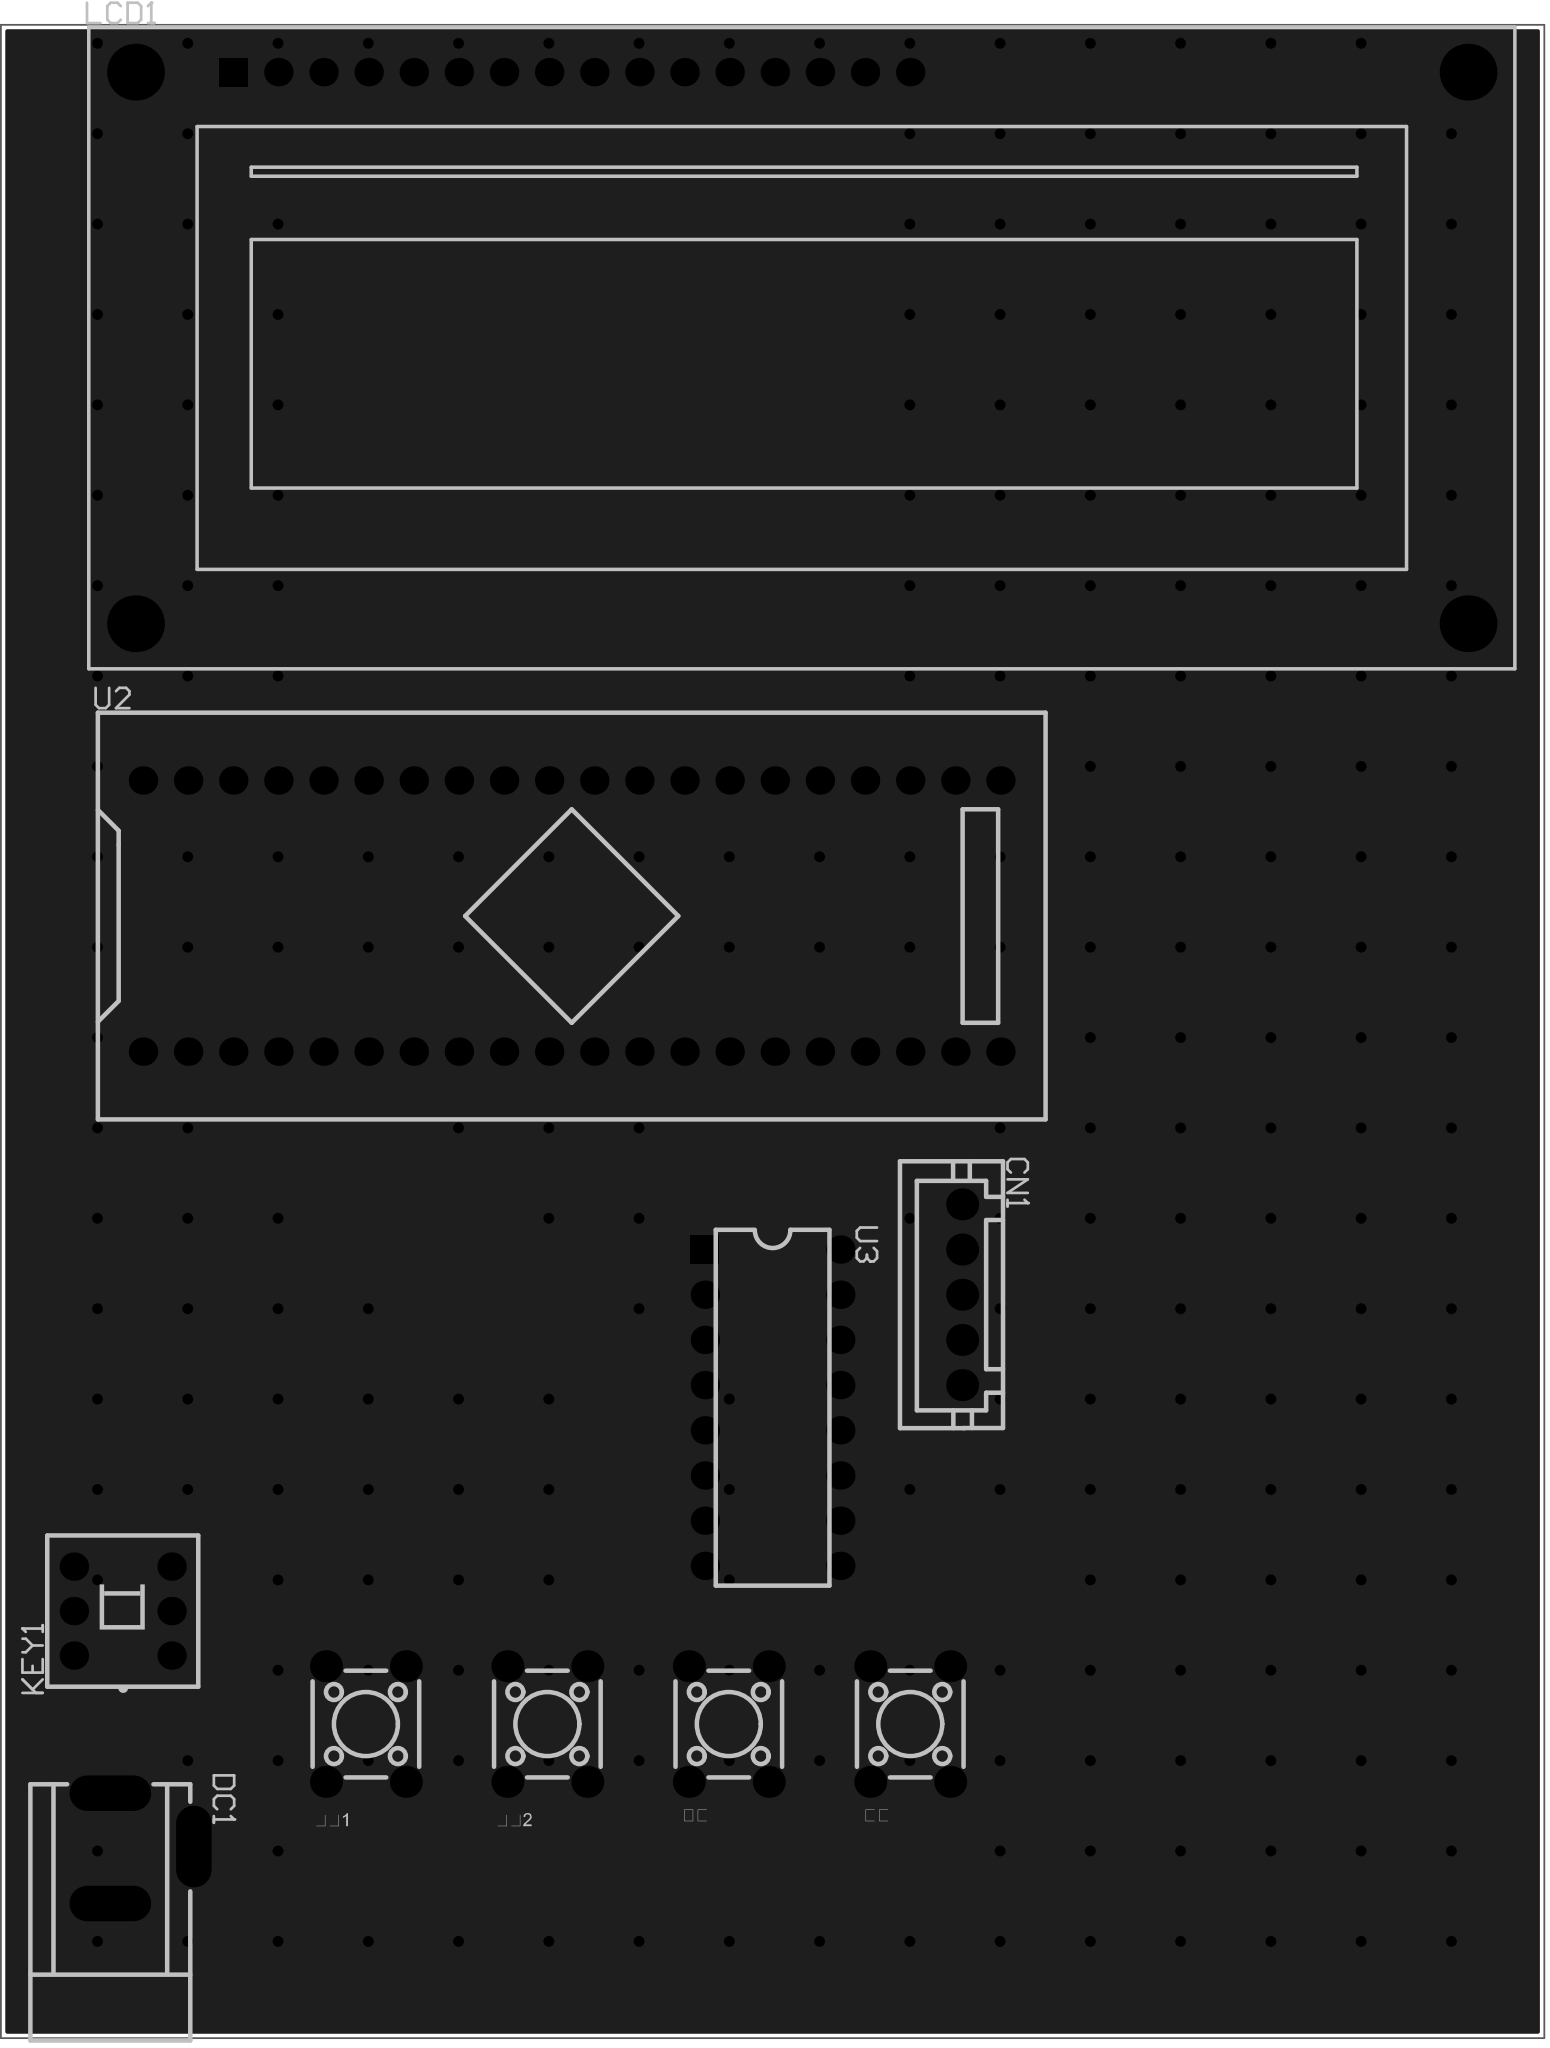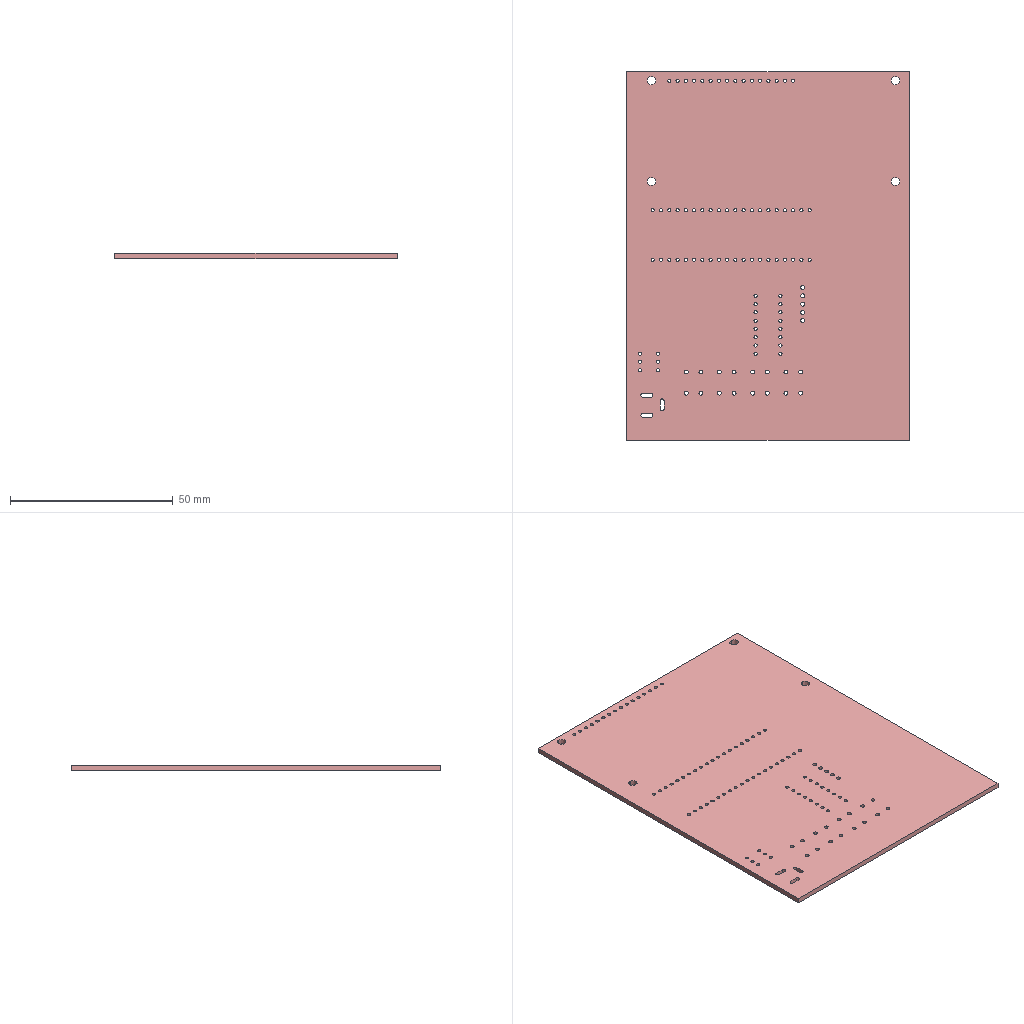Circuit board layout | Altium Designer | box 86.9 x 113.2 x 1.6 mm
Layer stack:
# Altium Designer layer stack of  (unit mm; dielectric type: 0 none, 1 core, 2 prepreg, 3 surface material)
index,name,kind,layer,copper_thickness_mm,dielectric_type,dielectric_thickness_mm,dielectric_material,dielectric_constant
0,Top Paste Mask Layer,other,,,,,,
1,Top Silkscreen Layer,other,,,,,,
2,Top Solder Mask Layer,dielectric,,,3,0.01,,3.3
3,Top Layer,copper,Top Layer,0.035,,,,
4,Dielectric1,dielectric,,,3,1.51,FR4,4.5
5,Bottom Layer,copper,Bottom Layer,0.035,,,,
6,Bottom Solder Mask Layer,dielectric,,,3,0.01,,3.3
7,Bottom Silkscreen Layer,other,,,,,,
8,Bottom Paste Mask Layer,other,,,,,,
# drill layer pairs: low layer,high layer
drill_pair,Top Layer,Bottom Layer
Part placement:
Designator,Comment,Layer,Footprint,Center-X(mm),Center-Y(mm),Rotation
CN1,XH2.54-5P,TopLayer,CONN-TH_5P-P2.54_C9900008095,137.668,131.064,270
U2,STM32F103C8T6-Card,TopLayer,CONN-TH_L53.3-W22.9_STM32F103C8T6-CARD,115.694,152.348,0
U3,ULN2003AN,TopLayer,DIP-16_L19.8-W6.5-P2.54-LS7.6-BL,127,124.714,270
LCD1,LMB162ADC,TopLayer,LCD1602,128.644,184.277,0
减速,,TopLayer,SW-TH_4P-L6.0-W6.0-P4.50-LS6.5,124.535,106.934,270
切换1,,TopLayer,SW-TH_4P-L6.0-W6.0-P4.50-LS6.5,104.11,106.934,270
切换2,,TopLayer,SW-TH_4P-L6.0-W6.0-P4.50-LS6.5,114.322,106.934,270
加速,,TopLayer,SW-TH_4P-L6.0-W6.0-P4.50-LS6.5,134.747,106.934,270
DC1,,TopLayer,DC-005_2.5,92.075,99.949,270
KEY1,Non-latching switch 8.5×8.5, silent,TopLayer,SW-TH_6P-L8.5-W8.5-P2.54,90.424,113.284,90
Pad and via stacks:
# Altium Designer via and pad stacks of  (unit mm). Each distinct definition once, with the count of objects using it.
# via: kind,start_layer,end_layer,hole_mm,diameter_mm,mode(0 simple;1 top-mid-bottom;2 full stack),diameter_per_layer,count,example_net
# pad: kind,layer,hole_mm,hole_type(0 round;1 square;2 slot),plating,top_size,top_shape(1 round;2 rect;3 octagon;9 rounded rect),mid_size,bottom_size,mode,footprint,size_per_layer,count,example
pad,Multi-Layer,1.2,0,plated,1.8x1.8,1,1.8x1.8,1.8x1.8,0,CONN-TH_5P-P2.54_C9900008095,,5,CN1.5
pad,Multi-Layer,1,0,plated,1.6x1.6,1,1.6x1.6,1.6x1.6,0,CONN-TH_L53.3-W22.9_STM32F103C8T6-CARD,,40,U2.1
pad,Multi-Layer,1,0,plated,1.6x1.6,1,1.6x1.6,1.6x1.6,0,DIP-16_L19.8-W6.5-P2.54-LS7.6-BL,,15,U3.16
pad,Multi-Layer,1,0,plated,1.6x1.6,2,1.6x1.6,1.6x1.6,0,DIP-16_L19.8-W6.5-P2.54-LS7.6-BL,,1,U3.1
pad,Multi-Layer,1,0,plated,1.6x1.6,1,1.6x1.6,1.6x1.6,0,LCD1602,,15,LCD1.16
pad,Multi-Layer,1,0,plated,1.6x1.6,2,1.6x1.6,1.6x1.6,0,LCD1602,,1,LCD1.1
pad,Multi-Layer,2.5,2,plated,3.2x3.2,1,3.2x3.2,3.2x3.2,0,LCD1602,,4,LCD1.0
pad,Multi-Layer,1.2,0,plated,1.8x1.8,1,1.8x1.8,1.8x1.8,0,SW-TH_4P-L6.0-W6.0-P4.50-LS6.5,,16,\u51CF\u901F.1
pad,Multi-Layer,1.2,2,plated,2x4.6,1,2x4.6,2x4.6,0,DC-005_2.5,,2,DC1.1
pad,Multi-Layer,1.2,2,plated,4.6x2,1,4.6x2,4.6x2,0,DC-005_2.5,,1,DC1.3
pad,Multi-Layer,1,0,plated,1.6x1.6,1,1.6x1.6,1.6x1.6,0,SW-TH_6P-L8.5-W8.5-P2.54,,6,KEY1.4
via,Top Layer,Bottom Layer,0.3048,0.61,0,,253,GND
Copper pours:
name,layer,net,type(0 solid;1 hatched;2 none)
Top Layer-GND,Top Layer,GND,0
Bottom Layer-GND,Bottom Layer,GND,0